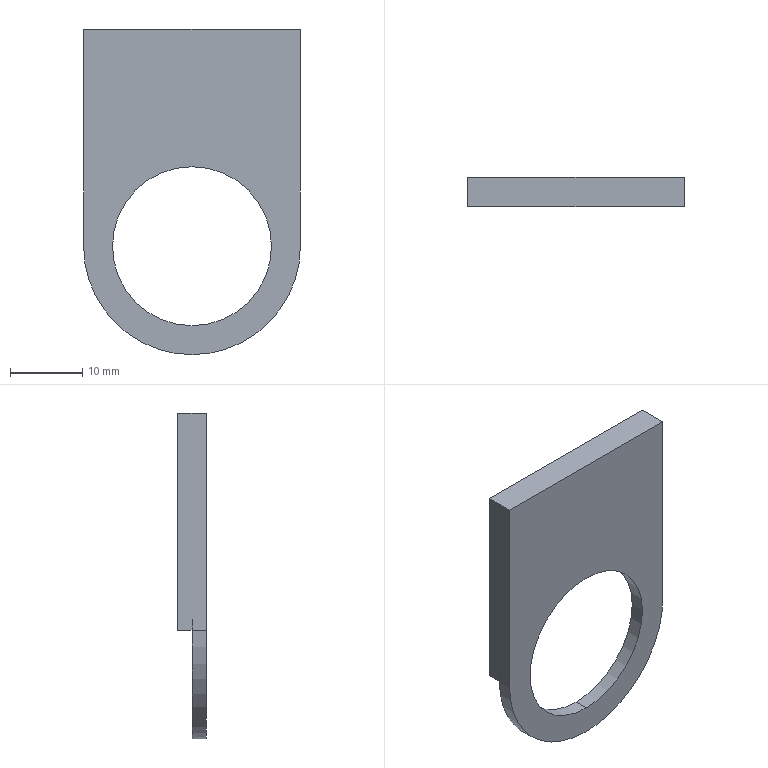Part | STEP file | Panel | 1 solid | 81 faces | box 30 x 4 x 45 mm | volume 2788 mm3 | plane 58 | spline 17 | cylinder 6 | commonest cylinder face diameters 30 x4 22 x2